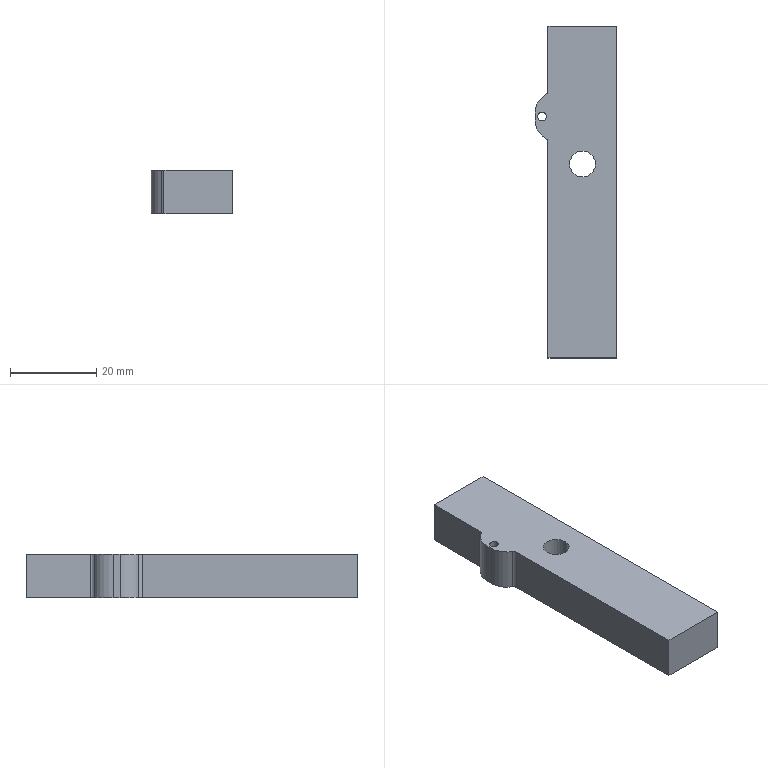Part | CATIA | 1 solid | 16 faces | box 19 x 77 x 10 mm | volume 12253 mm3 | plane 8 | cylinder 8 | commonest cylinder face diameters 2 x4 6 x2 10 x2
STEP:
#1=CARTESIAN_POINT('',(-35.495,19.,20.));
#2=VERTEX_POINT('',#1);
#3=CARTESIAN_POINT('',(-35.495,19.,30.));
#4=VERTEX_POINT('',#3);
#5=CARTESIAN_POINT('',(-35.495,19.,25.));
#6=DIRECTION('',(0.,0.,1.));
#7=VECTOR('',#6,1.);
#8=LINE('',#5,#7);
#9=EDGE_CURVE('',#2,#4,#8,.T.);
#10=ORIENTED_EDGE('',*,*,#9,.F.);
#11=CARTESIAN_POINT('',(-19.495,19.,20.));
#12=VERTEX_POINT('',#11);
#13=CARTESIAN_POINT('',(-27.495,19.,20.));
#14=DIRECTION('',(1.,0.,0.));
#15=VECTOR('',#14,1.);
#16=LINE('',#13,#15);
#17=EDGE_CURVE('',#2,#12,#16,.T.);
#18=ORIENTED_EDGE('',*,*,#17,.T.);
#19=CARTESIAN_POINT('',(-19.495,19.,30.));
#20=VERTEX_POINT('',#19);
#21=CARTESIAN_POINT('',(-19.495,19.,25.));
#22=DIRECTION('',(0.,0.,1.));
#23=VECTOR('',#22,1.);
#24=LINE('',#21,#23);
#25=EDGE_CURVE('',#12,#20,#24,.T.);
#26=ORIENTED_EDGE('',*,*,#25,.T.);
#27=CARTESIAN_POINT('',(-27.495,19.,30.));
#28=DIRECTION('',(1.,0.,0.));
#29=VECTOR('',#28,1.);
#30=LINE('',#27,#29);
#31=EDGE_CURVE('',#4,#20,#30,.T.);
#32=ORIENTED_EDGE('',*,*,#31,.F.);
#33=EDGE_LOOP('',(#10,#18,#26,#32));
#34=FACE_OUTER_BOUND('',#33,.T.);
#35=CARTESIAN_POINT('',(-35.495,19.,0.));
#36=DIRECTION('',(0.,-1.,0.));
#37=DIRECTION('',(1.,0.,0.));
#38=AXIS2_PLACEMENT_3D('',#35,#36,#37);
#39=PLANE('',#38);
#40=ADVANCED_FACE('',(#34),#39,.T.);
#41=CARTESIAN_POINT('',(-35.495,69.,20.));
#42=VERTEX_POINT('',#41);
#43=CARTESIAN_POINT('',(-35.495,44.,20.));
#44=DIRECTION('',(0.,-1.,0.));
#45=VECTOR('',#44,1.);
#46=LINE('',#43,#45);
#47=EDGE_CURVE('',#42,#2,#46,.T.);
#48=ORIENTED_EDGE('',*,*,#47,.T.);
#49=ORIENTED_EDGE('',*,*,#9,.T.);
#50=CARTESIAN_POINT('',(-35.495,69.,30.));
#51=VERTEX_POINT('',#50);
#52=CARTESIAN_POINT('',(-35.495,44.,30.));
#53=DIRECTION('',(0.,-1.,0.));
#54=VECTOR('',#53,1.);
#55=LINE('',#52,#54);
#56=EDGE_CURVE('',#51,#4,#55,.T.);
#57=ORIENTED_EDGE('',*,*,#56,.F.);
#58=CARTESIAN_POINT('',(-35.495,69.,25.));
#59=DIRECTION('',(0.,0.,-1.));
#60=VECTOR('',#59,1.);
#61=LINE('',#58,#60);
#62=EDGE_CURVE('',#51,#42,#61,.T.);
#63=ORIENTED_EDGE('',*,*,#62,.T.);
#64=EDGE_LOOP('',(#48,#49,#57,#63));
#65=FACE_OUTER_BOUND('',#64,.T.);
#66=CARTESIAN_POINT('',(-35.495,96.,0.));
#67=DIRECTION('',(-1.,0.,0.));
#68=DIRECTION('',(0.,-1.,0.));
#69=AXIS2_PLACEMENT_3D('',#66,#67,#68);
#70=PLANE('',#69);
#71=ADVANCED_FACE('',(#65),#70,.T.);
#72=CARTESIAN_POINT('',(-19.495,96.,20.));
#73=VERTEX_POINT('',#72);
#74=CARTESIAN_POINT('',(-35.495,96.,20.));
#75=VERTEX_POINT('',#74);
#76=CARTESIAN_POINT('',(-27.495,96.,20.));
#77=DIRECTION('',(1.,0.,0.));
#78=VECTOR('',#77,1.);
#79=LINE('',#76,#78);
#80=EDGE_CURVE('',#73,#75,#79,.F.);
#81=ORIENTED_EDGE('',*,*,#80,.F.);
#82=CARTESIAN_POINT('',(-19.495,57.5,20.));
#83=DIRECTION('',(0.,-1.,0.));
#84=VECTOR('',#83,1.);
#85=LINE('',#82,#84);
#86=EDGE_CURVE('',#12,#73,#85,.F.);
#87=ORIENTED_EDGE('',*,*,#86,.F.);
#88=ORIENTED_EDGE('',*,*,#17,.F.);
#89=ORIENTED_EDGE('',*,*,#47,.F.);
#90=CARTESIAN_POINT('',(-35.995,69.866,20.));
#91=VERTEX_POINT('',#90);
#92=CARTESIAN_POINT('',(-36.495,69.,20.));
#93=DIRECTION('',(0.,0.,1.));
#94=AXIS2_PLACEMENT_3D('',#92,#93,$);
#95=CIRCLE('',#94,1.);
#96=EDGE_CURVE('',#91,#42,#95,.F.);
#97=ORIENTED_EDGE('',*,*,#96,.F.);
#98=CARTESIAN_POINT('',(-38.495,74.196,20.));
#99=VERTEX_POINT('',#98);
#100=CARTESIAN_POINT('',(-33.495,74.196,20.));
#101=DIRECTION('',(0.,0.,1.));
#102=AXIS2_PLACEMENT_3D('',#100,#101,$);
#103=CIRCLE('',#102,5.);
#104=EDGE_CURVE('',#99,#91,#103,.T.);
#105=ORIENTED_EDGE('',*,*,#104,.F.);
#106=CARTESIAN_POINT('',(-38.495,75.804,20.));
#107=VERTEX_POINT('',#106);
#108=CARTESIAN_POINT('',(-38.495,75.,20.));
#109=DIRECTION('',(0.,-1.,0.));
#110=VECTOR('',#109,1.);
#111=LINE('',#108,#110);
#112=EDGE_CURVE('',#107,#99,#111,.T.);
#113=ORIENTED_EDGE('',*,*,#112,.F.);
#114=CARTESIAN_POINT('',(-35.995,80.134,20.));
#115=VERTEX_POINT('',#114);
#116=CARTESIAN_POINT('',(-33.495,75.804,20.));
#117=DIRECTION('',(0.,0.,1.));
#118=AXIS2_PLACEMENT_3D('',#116,#117,$);
#119=CIRCLE('',#118,5.);
#120=EDGE_CURVE('',#115,#107,#119,.T.);
#121=ORIENTED_EDGE('',*,*,#120,.F.);
#122=CARTESIAN_POINT('',(-35.495,81.,20.));
#123=VERTEX_POINT('',#122);
#124=CARTESIAN_POINT('',(-36.495,81.,20.));
#125=DIRECTION('',(0.,0.,1.));
#126=AXIS2_PLACEMENT_3D('',#124,#125,$);
#127=CIRCLE('',#126,1.);
#128=EDGE_CURVE('',#123,#115,#127,.F.);
#129=ORIENTED_EDGE('',*,*,#128,.F.);
#130=CARTESIAN_POINT('',(-35.495,88.5,20.));
#131=DIRECTION('',(0.,-1.,0.));
#132=VECTOR('',#131,1.);
#133=LINE('',#130,#132);
#134=EDGE_CURVE('',#75,#123,#133,.T.);
#135=ORIENTED_EDGE('',*,*,#134,.F.);
#136=EDGE_LOOP('',(#81,#87,#88,#89,#97,#105,#113,#121,#129,#135));
#137=FACE_OUTER_BOUND('',#136,.T.);
#138=CARTESIAN_POINT('',(-30.495,64.,20.));
#139=VERTEX_POINT('',#138);
#140=CARTESIAN_POINT('',(-24.495,64.,20.));
#141=VERTEX_POINT('',#140);
#142=CARTESIAN_POINT('',(-27.495,64.,20.));
#143=DIRECTION('',(0.,0.,1.));
#144=AXIS2_PLACEMENT_3D('',#142,#143,$);
#145=CIRCLE('',#144,3.);
#146=EDGE_CURVE('',#139,#141,#145,.T.);
#147=ORIENTED_EDGE('',*,*,#146,.T.);
#148=CARTESIAN_POINT('',(-27.495,64.,20.));
#149=DIRECTION('',(0.,0.,1.));
#150=AXIS2_PLACEMENT_3D('',#148,#149,$);
#151=CIRCLE('',#150,3.);
#152=EDGE_CURVE('',#141,#139,#151,.T.);
#153=ORIENTED_EDGE('',*,*,#152,.T.);
#154=EDGE_LOOP('',(#147,#153));
#155=FACE_BOUND('',#154,.T.);
#156=CARTESIAN_POINT('',(-37.884,75.,20.));
#157=VERTEX_POINT('',#156);
#158=CARTESIAN_POINT('',(-35.884,75.,20.));
#159=VERTEX_POINT('',#158);
#160=CARTESIAN_POINT('',(-36.884,75.,20.));
#161=DIRECTION('',(0.,0.,1.));
#162=AXIS2_PLACEMENT_3D('',#160,#161,$);
#163=CIRCLE('',#162,1.);
#164=EDGE_CURVE('',#157,#159,#163,.T.);
#165=ORIENTED_EDGE('',*,*,#164,.T.);
#166=CARTESIAN_POINT('',(-36.884,75.,20.));
#167=DIRECTION('',(0.,0.,1.));
#168=AXIS2_PLACEMENT_3D('',#166,#167,$);
#169=CIRCLE('',#168,1.);
#170=EDGE_CURVE('',#159,#157,#169,.T.);
#171=ORIENTED_EDGE('',*,*,#170,.T.);
#172=EDGE_LOOP('',(#165,#171));
#173=FACE_BOUND('',#172,.T.);
#174=CARTESIAN_POINT('',(0.,0.,20.));
#175=DIRECTION('',(0.,0.,1.));
#176=DIRECTION('',(1.,0.,0.));
#177=AXIS2_PLACEMENT_3D('',#174,#175,#176);
#178=PLANE('',#177);
#179=ADVANCED_FACE('',(#137,#155,#173),#178,.F.);
#180=ORIENTED_EDGE('',*,*,#25,.F.);
#181=ORIENTED_EDGE('',*,*,#86,.T.);
#182=CARTESIAN_POINT('',(-19.495,96.,30.));
#183=VERTEX_POINT('',#182);
#184=CARTESIAN_POINT('',(-19.495,96.,25.));
#185=DIRECTION('',(0.,0.,1.));
#186=VECTOR('',#185,1.);
#187=LINE('',#184,#186);
#188=EDGE_CURVE('',#73,#183,#187,.T.);
#189=ORIENTED_EDGE('',*,*,#188,.T.);
#190=CARTESIAN_POINT('',(-19.495,57.5,30.));
#191=DIRECTION('',(0.,-1.,0.));
#192=VECTOR('',#191,1.);
#193=LINE('',#190,#192);
#194=EDGE_CURVE('',#20,#183,#193,.F.);
#195=ORIENTED_EDGE('',*,*,#194,.F.);
#196=EDGE_LOOP('',(#180,#181,#189,#195));
#197=FACE_OUTER_BOUND('',#196,.T.);
#198=CARTESIAN_POINT('',(-19.495,96.,0.));
#199=DIRECTION('',(-1.,0.,0.));
#200=DIRECTION('',(0.,-1.,0.));
#201=AXIS2_PLACEMENT_3D('',#198,#199,#200);
#202=PLANE('',#201);
#203=ADVANCED_FACE('',(#197),#202,.F.);
#204=CARTESIAN_POINT('',(-35.495,96.,30.));
#205=VERTEX_POINT('',#204);
#206=CARTESIAN_POINT('',(-35.495,81.,30.));
#207=VERTEX_POINT('',#206);
#208=CARTESIAN_POINT('',(-35.495,88.5,30.));
#209=DIRECTION('',(0.,-1.,0.));
#210=VECTOR('',#209,1.);
#211=LINE('',#208,#210);
#212=EDGE_CURVE('',#205,#207,#211,.T.);
#213=ORIENTED_EDGE('',*,*,#212,.T.);
#214=CARTESIAN_POINT('',(-35.995,80.134,30.));
#215=VERTEX_POINT('',#214);
#216=CARTESIAN_POINT('',(-36.495,81.,30.));
#217=DIRECTION('',(0.,0.,1.));
#218=AXIS2_PLACEMENT_3D('',#216,#217,$);
#219=CIRCLE('',#218,1.);
#220=EDGE_CURVE('',#207,#215,#219,.F.);
#221=ORIENTED_EDGE('',*,*,#220,.T.);
#222=CARTESIAN_POINT('',(-38.495,75.804,30.));
#223=VERTEX_POINT('',#222);
#224=CARTESIAN_POINT('',(-33.495,75.804,30.));
#225=DIRECTION('',(0.,0.,1.));
#226=AXIS2_PLACEMENT_3D('',#224,#225,$);
#227=CIRCLE('',#226,5.);
#228=EDGE_CURVE('',#215,#223,#227,.T.);
#229=ORIENTED_EDGE('',*,*,#228,.T.);
#230=CARTESIAN_POINT('',(-38.495,74.196,30.));
#231=VERTEX_POINT('',#230);
#232=CARTESIAN_POINT('',(-38.495,75.,30.));
#233=DIRECTION('',(0.,-1.,0.));
#234=VECTOR('',#233,1.);
#235=LINE('',#232,#234);
#236=EDGE_CURVE('',#223,#231,#235,.T.);
#237=ORIENTED_EDGE('',*,*,#236,.T.);
#238=CARTESIAN_POINT('',(-35.995,69.866,30.));
#239=VERTEX_POINT('',#238);
#240=CARTESIAN_POINT('',(-33.495,74.196,30.));
#241=DIRECTION('',(0.,0.,1.));
#242=AXIS2_PLACEMENT_3D('',#240,#241,$);
#243=CIRCLE('',#242,5.);
#244=EDGE_CURVE('',#231,#239,#243,.T.);
#245=ORIENTED_EDGE('',*,*,#244,.T.);
#246=CARTESIAN_POINT('',(-36.495,69.,30.));
#247=DIRECTION('',(0.,0.,1.));
#248=AXIS2_PLACEMENT_3D('',#246,#247,$);
#249=CIRCLE('',#248,1.);
#250=EDGE_CURVE('',#239,#51,#249,.F.);
#251=ORIENTED_EDGE('',*,*,#250,.T.);
#252=ORIENTED_EDGE('',*,*,#56,.T.);
#253=ORIENTED_EDGE('',*,*,#31,.T.);
#254=ORIENTED_EDGE('',*,*,#194,.T.);
#255=CARTESIAN_POINT('',(-27.495,96.,30.));
#256=DIRECTION('',(1.,0.,0.));
#257=VECTOR('',#256,1.);
#258=LINE('',#255,#257);
#259=EDGE_CURVE('',#183,#205,#258,.F.);
#260=ORIENTED_EDGE('',*,*,#259,.T.);
#261=EDGE_LOOP('',(#213,#221,#229,#237,#245,#251,#252,#253,#254,#260));
#262=FACE_OUTER_BOUND('',#261,.T.);
#263=CARTESIAN_POINT('',(-24.495,64.,30.));
#264=VERTEX_POINT('',#263);
#265=CARTESIAN_POINT('',(-30.495,64.,30.));
#266=VERTEX_POINT('',#265);
#267=CARTESIAN_POINT('',(-27.495,64.,30.));
#268=DIRECTION('',(0.,0.,1.));
#269=AXIS2_PLACEMENT_3D('',#267,#268,$);
#270=CIRCLE('',#269,3.);
#271=EDGE_CURVE('',#264,#266,#270,.T.);
#272=ORIENTED_EDGE('',*,*,#271,.F.);
#273=CARTESIAN_POINT('',(-27.495,64.,30.));
#274=DIRECTION('',(0.,0.,1.));
#275=AXIS2_PLACEMENT_3D('',#273,#274,$);
#276=CIRCLE('',#275,3.);
#277=EDGE_CURVE('',#266,#264,#276,.T.);
#278=ORIENTED_EDGE('',*,*,#277,.F.);
#279=EDGE_LOOP('',(#272,#278));
#280=FACE_BOUND('',#279,.T.);
#281=CARTESIAN_POINT('',(-35.884,75.,30.));
#282=VERTEX_POINT('',#281);
#283=CARTESIAN_POINT('',(-37.884,75.,30.));
#284=VERTEX_POINT('',#283);
#285=CARTESIAN_POINT('',(-36.884,75.,30.));
#286=DIRECTION('',(0.,0.,1.));
#287=AXIS2_PLACEMENT_3D('',#285,#286,$);
#288=CIRCLE('',#287,1.);
#289=EDGE_CURVE('',#282,#284,#288,.T.);
#290=ORIENTED_EDGE('',*,*,#289,.F.);
#291=CARTESIAN_POINT('',(-36.884,75.,30.));
#292=DIRECTION('',(0.,0.,1.));
#293=AXIS2_PLACEMENT_3D('',#291,#292,$);
#294=CIRCLE('',#293,1.);
#295=EDGE_CURVE('',#284,#282,#294,.T.);
#296=ORIENTED_EDGE('',*,*,#295,.F.);
#297=EDGE_LOOP('',(#290,#296));
#298=FACE_BOUND('',#297,.T.);
#299=CARTESIAN_POINT('',(0.,0.,30.));
#300=DIRECTION('',(0.,0.,1.));
#301=DIRECTION('',(1.,0.,0.));
#302=AXIS2_PLACEMENT_3D('',#299,#300,#301);
#303=PLANE('',#302);
#304=ADVANCED_FACE('',(#262,#280,#298),#303,.T.);
#305=ORIENTED_EDGE('',*,*,#96,.T.);
#306=ORIENTED_EDGE('',*,*,#62,.F.);
#307=ORIENTED_EDGE('',*,*,#250,.F.);
#308=CARTESIAN_POINT('',(-35.995,69.866,25.));
#309=DIRECTION('',(0.,0.,1.));
#310=VECTOR('',#309,1.);
#311=LINE('',#308,#310);
#312=EDGE_CURVE('',#239,#91,#311,.F.);
#313=ORIENTED_EDGE('',*,*,#312,.T.);
#314=EDGE_LOOP('',(#305,#306,#307,#313));
#315=FACE_OUTER_BOUND('',#314,.T.);
#316=CARTESIAN_POINT('',(-36.495,69.,25.));
#317=DIRECTION('',(0.,0.,1.));
#318=DIRECTION('',(1.,0.,0.));
#319=AXIS2_PLACEMENT_3D('',#316,#317,#318);
#320=CYLINDRICAL_SURFACE('',#319,1.);
#321=ADVANCED_FACE('',(#315),#320,.F.);
#322=ORIENTED_EDGE('',*,*,#188,.F.);
#323=ORIENTED_EDGE('',*,*,#80,.T.);
#324=CARTESIAN_POINT('',(-35.495,96.,25.));
#325=DIRECTION('',(0.,0.,1.));
#326=VECTOR('',#325,1.);
#327=LINE('',#324,#326);
#328=EDGE_CURVE('',#75,#205,#327,.T.);
#329=ORIENTED_EDGE('',*,*,#328,.T.);
#330=ORIENTED_EDGE('',*,*,#259,.F.);
#331=EDGE_LOOP('',(#322,#323,#329,#330));
#332=FACE_OUTER_BOUND('',#331,.T.);
#333=CARTESIAN_POINT('',(-35.495,96.,0.));
#334=DIRECTION('',(0.,-1.,0.));
#335=DIRECTION('',(1.,0.,0.));
#336=AXIS2_PLACEMENT_3D('',#333,#334,#335);
#337=PLANE('',#336);
#338=ADVANCED_FACE('',(#332),#337,.F.);
#339=ORIENTED_EDGE('',*,*,#104,.T.);
#340=ORIENTED_EDGE('',*,*,#312,.F.);
#341=ORIENTED_EDGE('',*,*,#244,.F.);
#342=CARTESIAN_POINT('',(-38.495,74.196,25.));
#343=DIRECTION('',(0.,0.,1.));
#344=VECTOR('',#343,1.);
#345=LINE('',#342,#344);
#346=EDGE_CURVE('',#231,#99,#345,.F.);
#347=ORIENTED_EDGE('',*,*,#346,.T.);
#348=EDGE_LOOP('',(#339,#340,#341,#347));
#349=FACE_OUTER_BOUND('',#348,.T.);
#350=CARTESIAN_POINT('',(-33.495,74.196,25.));
#351=DIRECTION('',(0.,0.,1.));
#352=DIRECTION('',(-1.,0.,0.));
#353=AXIS2_PLACEMENT_3D('',#350,#351,#352);
#354=CYLINDRICAL_SURFACE('',#353,5.);
#355=ADVANCED_FACE('',(#349),#354,.T.);
#356=ORIENTED_EDGE('',*,*,#112,.T.);
#357=ORIENTED_EDGE('',*,*,#346,.F.);
#358=ORIENTED_EDGE('',*,*,#236,.F.);
#359=CARTESIAN_POINT('',(-38.495,75.804,25.));
#360=DIRECTION('',(0.,0.,1.));
#361=VECTOR('',#360,1.);
#362=LINE('',#359,#361);
#363=EDGE_CURVE('',#223,#107,#362,.F.);
#364=ORIENTED_EDGE('',*,*,#363,.T.);
#365=EDGE_LOOP('',(#356,#357,#358,#364));
#366=FACE_OUTER_BOUND('',#365,.T.);
#367=CARTESIAN_POINT('',(-38.495,75.804,30.));
#368=DIRECTION('',(1.,0.,0.));
#369=DIRECTION('',(0.,-1.,0.));
#370=AXIS2_PLACEMENT_3D('',#367,#368,#369);
#371=PLANE('',#370);
#372=ADVANCED_FACE('',(#366),#371,.F.);
#373=ORIENTED_EDGE('',*,*,#120,.T.);
#374=ORIENTED_EDGE('',*,*,#363,.F.);
#375=ORIENTED_EDGE('',*,*,#228,.F.);
#376=CARTESIAN_POINT('',(-35.995,80.134,25.));
#377=DIRECTION('',(0.,0.,1.));
#378=VECTOR('',#377,1.);
#379=LINE('',#376,#378);
#380=EDGE_CURVE('',#215,#115,#379,.F.);
#381=ORIENTED_EDGE('',*,*,#380,.T.);
#382=EDGE_LOOP('',(#373,#374,#375,#381));
#383=FACE_OUTER_BOUND('',#382,.T.);
#384=CARTESIAN_POINT('',(-33.495,75.804,25.));
#385=DIRECTION('',(0.,0.,1.));
#386=DIRECTION('',(-0.5,0.866,0.));
#387=AXIS2_PLACEMENT_3D('',#384,#385,#386);
#388=CYLINDRICAL_SURFACE('',#387,5.);
#389=ADVANCED_FACE('',(#383),#388,.T.);
#390=ORIENTED_EDGE('',*,*,#128,.T.);
#391=ORIENTED_EDGE('',*,*,#380,.F.);
#392=ORIENTED_EDGE('',*,*,#220,.F.);
#393=CARTESIAN_POINT('',(-35.495,81.,25.));
#394=DIRECTION('',(0.,0.,1.));
#395=VECTOR('',#394,1.);
#396=LINE('',#393,#395);
#397=EDGE_CURVE('',#207,#123,#396,.F.);
#398=ORIENTED_EDGE('',*,*,#397,.T.);
#399=EDGE_LOOP('',(#390,#391,#392,#398));
#400=FACE_OUTER_BOUND('',#399,.T.);
#401=CARTESIAN_POINT('',(-36.495,81.,25.));
#402=DIRECTION('',(0.,0.,1.));
#403=DIRECTION('',(0.5,-0.866,0.));
#404=AXIS2_PLACEMENT_3D('',#401,#402,#403);
#405=CYLINDRICAL_SURFACE('',#404,1.);
#406=ADVANCED_FACE('',(#400),#405,.F.);
#407=ORIENTED_EDGE('',*,*,#212,.F.);
#408=ORIENTED_EDGE('',*,*,#328,.F.);
#409=ORIENTED_EDGE('',*,*,#134,.T.);
#410=ORIENTED_EDGE('',*,*,#397,.F.);
#411=EDGE_LOOP('',(#407,#408,#409,#410));
#412=FACE_OUTER_BOUND('',#411,.T.);
#413=ADVANCED_FACE('',(#412),#70,.T.);
#414=CARTESIAN_POINT('',(-24.495,64.,25.));
#415=DIRECTION('',(0.,0.,1.));
#416=VECTOR('',#415,1.);
#417=LINE('',#414,#416);
#418=EDGE_CURVE('',#264,#141,#417,.F.);
#419=ORIENTED_EDGE('',*,*,#418,.T.);
#420=ORIENTED_EDGE('',*,*,#146,.F.);
#421=CARTESIAN_POINT('',(-30.495,64.,25.));
#422=DIRECTION('',(0.,0.,1.));
#423=VECTOR('',#422,1.);
#424=LINE('',#421,#423);
#425=EDGE_CURVE('',#266,#139,#424,.F.);
#426=ORIENTED_EDGE('',*,*,#425,.F.);
#427=ORIENTED_EDGE('',*,*,#277,.T.);
#428=EDGE_LOOP('',(#419,#420,#426,#427));
#429=FACE_OUTER_BOUND('',#428,.T.);
#430=CARTESIAN_POINT('',(-27.495,64.,25.));
#431=DIRECTION('',(0.,0.,1.));
#432=DIRECTION('',(-1.,0.,0.));
#433=AXIS2_PLACEMENT_3D('',#430,#431,#432);
#434=CYLINDRICAL_SURFACE('',#433,3.);
#435=ADVANCED_FACE('',(#429),#434,.F.);
#436=ORIENTED_EDGE('',*,*,#425,.T.);
#437=ORIENTED_EDGE('',*,*,#152,.F.);
#438=ORIENTED_EDGE('',*,*,#418,.F.);
#439=ORIENTED_EDGE('',*,*,#271,.T.);
#440=EDGE_LOOP('',(#436,#437,#438,#439));
#441=FACE_OUTER_BOUND('',#440,.T.);
#442=CARTESIAN_POINT('',(-27.495,64.,25.));
#443=DIRECTION('',(0.,0.,1.));
#444=DIRECTION('',(1.,0.,0.));
#445=AXIS2_PLACEMENT_3D('',#442,#443,#444);
#446=CYLINDRICAL_SURFACE('',#445,3.);
#447=ADVANCED_FACE('',(#441),#446,.F.);
#448=CARTESIAN_POINT('',(-37.884,75.,25.));
#449=DIRECTION('',(0.,0.,1.));
#450=VECTOR('',#449,1.);
#451=LINE('',#448,#450);
#452=EDGE_CURVE('',#284,#157,#451,.F.);
#453=ORIENTED_EDGE('',*,*,#452,.F.);
#454=ORIENTED_EDGE('',*,*,#295,.T.);
#455=CARTESIAN_POINT('',(-35.884,75.,25.));
#456=DIRECTION('',(0.,0.,1.));
#457=VECTOR('',#456,1.);
#458=LINE('',#455,#457);
#459=EDGE_CURVE('',#282,#159,#458,.F.);
#460=ORIENTED_EDGE('',*,*,#459,.T.);
#461=ORIENTED_EDGE('',*,*,#164,.F.);
#462=EDGE_LOOP('',(#453,#454,#460,#461));
#463=FACE_OUTER_BOUND('',#462,.T.);
#464=CARTESIAN_POINT('',(-36.884,75.,25.));
#465=DIRECTION('',(0.,0.,1.));
#466=DIRECTION('',(-1.,0.,0.));
#467=AXIS2_PLACEMENT_3D('',#464,#465,#466);
#468=CYLINDRICAL_SURFACE('',#467,1.);
#469=ADVANCED_FACE('',(#463),#468,.F.);
#470=ORIENTED_EDGE('',*,*,#459,.F.);
#471=ORIENTED_EDGE('',*,*,#289,.T.);
#472=ORIENTED_EDGE('',*,*,#452,.T.);
#473=ORIENTED_EDGE('',*,*,#170,.F.);
#474=EDGE_LOOP('',(#470,#471,#472,#473));
#475=FACE_OUTER_BOUND('',#474,.T.);
#476=CARTESIAN_POINT('',(-36.884,75.,25.));
#477=DIRECTION('',(0.,0.,1.));
#478=DIRECTION('',(1.,0.,0.));
#479=AXIS2_PLACEMENT_3D('',#476,#477,#478);
#480=CYLINDRICAL_SURFACE('',#479,1.);
#481=ADVANCED_FACE('',(#475),#480,.F.);
#482=CLOSED_SHELL('',(#40,#71,#179,#203,#304,#321,#338,#355,#372,#389,#406,#413,#435,#447,#469,#481));
#483=MANIFOLD_SOLID_BREP('',#482);
#484=(LENGTH_UNIT()NAMED_UNIT(*)SI_UNIT(.MILLI.,.METRE.));
#485=UNCERTAINTY_MEASURE_WITH_UNIT(LENGTH_MEASURE(0.005),#484,'','');
#486=(NAMED_UNIT(*)PLANE_ANGLE_UNIT()SI_UNIT($,.RADIAN.));
#487=(NAMED_UNIT(*)SI_UNIT($,.STERADIAN.)SOLID_ANGLE_UNIT());
#488=(GEOMETRIC_REPRESENTATION_CONTEXT(3)GLOBAL_UNCERTAINTY_ASSIGNED_CONTEXT((#485))GLOBAL_UNIT_ASSIGNED_CONTEXT((#484,#486,#487))REPRESENTATION_CONTEXT('',''));
#489=ADVANCED_BREP_SHAPE_REPRESENTATION('',(#483),#488);